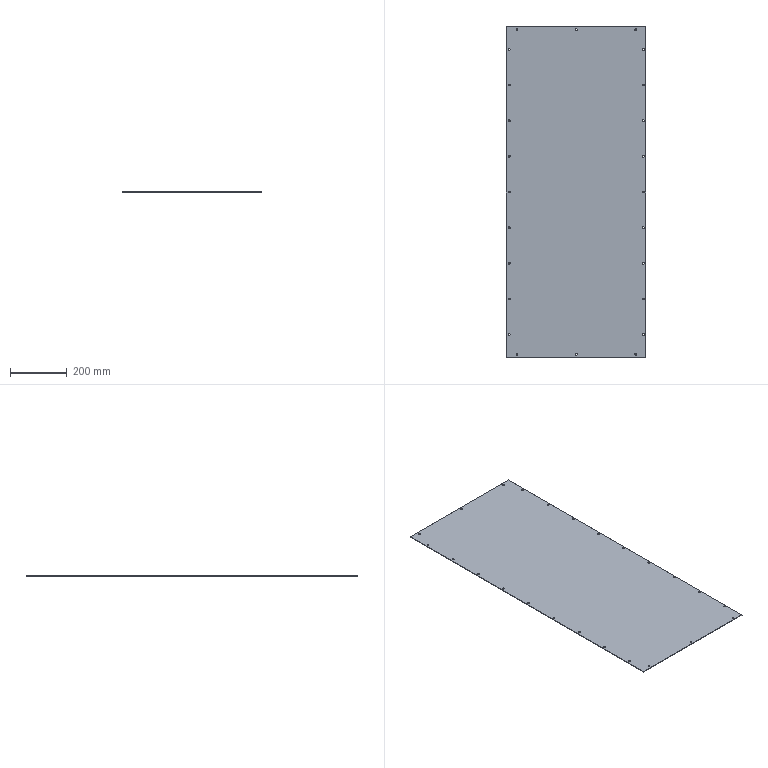Part | SolidWorks | 1 solid | 54 faces | box 492 x 1168 x 2 mm | volume 1147719 mm3 | cylinder 48 | plane 6 | commonest cylinder face diameters 6.5 x48